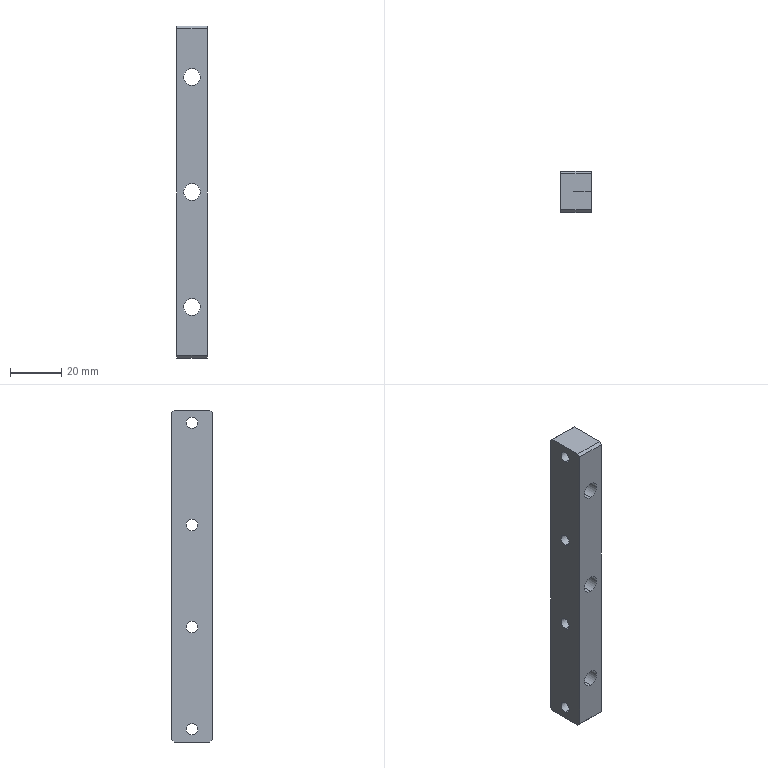Part | SolidWorks | features BaseBody 1 | 1 solid | 45 faces | box 12 x 16 x 130 mm | volume 19917 mm3 | cylinder 28 | plane 17 | commonest cylinder face diameters 4.5 x8 9 x8 6.6 x6 11 x6
STEP:
#1=CARTESIAN_POINT('',(-724.66,-691.086,-337.569));
#2=VERTEX_POINT('',#1);
#3=CARTESIAN_POINT('',(-724.66,-691.086,-333.069));
#4=VERTEX_POINT('',#3);
#5=CARTESIAN_POINT('',(-724.66,-691.086,-335.319));
#6=DIRECTION('',(-1.,0.,0.));
#7=DIRECTION('',(0.,0.,-1.));
#8=AXIS2_PLACEMENT_3D('',#5,#6,#7);
#9=CIRCLE('',#8,2.25);
#10=EDGE_CURVE('',#2,#4,#9,.T.);
#11=ORIENTED_EDGE('',*,*,#10,.T.);
#12=CARTESIAN_POINT('',(-719.66,-691.086,-333.069));
#13=VERTEX_POINT('',#12);
#14=CARTESIAN_POINT('',(-712.66,-691.086,-333.069));
#15=DIRECTION('',(1.,0.,0.));
#16=VECTOR('',#15,1000.);
#17=LINE('',#14,#16);
#18=EDGE_CURVE('',#4,#13,#17,.T.);
#19=ORIENTED_EDGE('',*,*,#18,.T.);
#20=CARTESIAN_POINT('',(-719.66,-691.086,-337.569));
#21=VERTEX_POINT('',#20);
#22=CARTESIAN_POINT('',(-719.66,-691.086,-335.319));
#23=DIRECTION('',(-1.,0.,0.));
#24=DIRECTION('',(0.,0.,-1.));
#25=AXIS2_PLACEMENT_3D('',#22,#23,#24);
#26=CIRCLE('',#25,2.25);
#27=EDGE_CURVE('',#21,#13,#26,.T.);
#28=ORIENTED_EDGE('',*,*,#27,.F.);
#29=CARTESIAN_POINT('',(-712.66,-691.086,-337.569));
#30=DIRECTION('',(1.,0.,0.));
#31=VECTOR('',#30,1000.);
#32=LINE('',#29,#31);
#33=EDGE_CURVE('',#2,#21,#32,.T.);
#34=ORIENTED_EDGE('',*,*,#33,.F.);
#35=EDGE_LOOP('',(#11,#19,#28,#34));
#36=FACE_OUTER_BOUND('',#35,.T.);
#37=CARTESIAN_POINT('',(-712.66,-691.086,-335.319));
#38=DIRECTION('',(1.,0.,0.));
#39=DIRECTION('',(0.,0.,-1.));
#40=AXIS2_PLACEMENT_3D('',#37,#38,#39);
#41=CYLINDRICAL_SURFACE('',#40,2.25);
#42=ADVANCED_FACE('',(#36),#41,.F.);
#43=CARTESIAN_POINT('',(-724.66,-691.086,-377.569));
#44=VERTEX_POINT('',#43);
#45=CARTESIAN_POINT('',(-724.66,-691.086,-373.069));
#46=VERTEX_POINT('',#45);
#47=CARTESIAN_POINT('',(-724.66,-691.086,-375.319));
#48=DIRECTION('',(-1.,0.,0.));
#49=DIRECTION('',(0.,0.,-1.));
#50=AXIS2_PLACEMENT_3D('',#47,#48,#49);
#51=CIRCLE('',#50,2.25);
#52=EDGE_CURVE('',#44,#46,#51,.T.);
#53=ORIENTED_EDGE('',*,*,#52,.T.);
#54=CARTESIAN_POINT('',(-719.66,-691.086,-373.069));
#55=VERTEX_POINT('',#54);
#56=CARTESIAN_POINT('',(-712.66,-691.086,-373.069));
#57=DIRECTION('',(1.,0.,0.));
#58=VECTOR('',#57,1000.);
#59=LINE('',#56,#58);
#60=EDGE_CURVE('',#46,#55,#59,.T.);
#61=ORIENTED_EDGE('',*,*,#60,.T.);
#62=CARTESIAN_POINT('',(-719.66,-691.086,-377.569));
#63=VERTEX_POINT('',#62);
#64=CARTESIAN_POINT('',(-719.66,-691.086,-375.319));
#65=DIRECTION('',(-1.,0.,0.));
#66=DIRECTION('',(0.,0.,-1.));
#67=AXIS2_PLACEMENT_3D('',#64,#65,#66);
#68=CIRCLE('',#67,2.25);
#69=EDGE_CURVE('',#63,#55,#68,.T.);
#70=ORIENTED_EDGE('',*,*,#69,.F.);
#71=CARTESIAN_POINT('',(-712.66,-691.086,-377.569));
#72=DIRECTION('',(1.,0.,0.));
#73=VECTOR('',#72,1000.);
#74=LINE('',#71,#73);
#75=EDGE_CURVE('',#44,#63,#74,.T.);
#76=ORIENTED_EDGE('',*,*,#75,.F.);
#77=EDGE_LOOP('',(#53,#61,#70,#76));
#78=FACE_OUTER_BOUND('',#77,.T.);
#79=CARTESIAN_POINT('',(-712.66,-691.086,-375.319));
#80=DIRECTION('',(1.,0.,0.));
#81=DIRECTION('',(0.,0.,-1.));
#82=AXIS2_PLACEMENT_3D('',#79,#80,#81);
#83=CYLINDRICAL_SURFACE('',#82,2.25);
#84=ADVANCED_FACE('',(#78),#83,.F.);
#85=CARTESIAN_POINT('',(-724.66,-691.086,-417.569));
#86=VERTEX_POINT('',#85);
#87=CARTESIAN_POINT('',(-724.66,-691.086,-413.069));
#88=VERTEX_POINT('',#87);
#89=CARTESIAN_POINT('',(-724.66,-691.086,-415.319));
#90=DIRECTION('',(-1.,0.,0.));
#91=DIRECTION('',(0.,0.,-1.));
#92=AXIS2_PLACEMENT_3D('',#89,#90,#91);
#93=CIRCLE('',#92,2.25);
#94=EDGE_CURVE('',#86,#88,#93,.T.);
#95=ORIENTED_EDGE('',*,*,#94,.T.);
#96=CARTESIAN_POINT('',(-719.66,-691.086,-413.069));
#97=VERTEX_POINT('',#96);
#98=CARTESIAN_POINT('',(-712.66,-691.086,-413.069));
#99=DIRECTION('',(1.,0.,0.));
#100=VECTOR('',#99,1000.);
#101=LINE('',#98,#100);
#102=EDGE_CURVE('',#88,#97,#101,.T.);
#103=ORIENTED_EDGE('',*,*,#102,.T.);
#104=CARTESIAN_POINT('',(-719.66,-691.086,-417.569));
#105=VERTEX_POINT('',#104);
#106=CARTESIAN_POINT('',(-719.66,-691.086,-415.319));
#107=DIRECTION('',(-1.,0.,0.));
#108=DIRECTION('',(0.,0.,-1.));
#109=AXIS2_PLACEMENT_3D('',#106,#107,#108);
#110=CIRCLE('',#109,2.25);
#111=EDGE_CURVE('',#105,#97,#110,.T.);
#112=ORIENTED_EDGE('',*,*,#111,.F.);
#113=CARTESIAN_POINT('',(-712.66,-691.086,-417.569));
#114=DIRECTION('',(1.,0.,0.));
#115=VECTOR('',#114,1000.);
#116=LINE('',#113,#115);
#117=EDGE_CURVE('',#86,#105,#116,.T.);
#118=ORIENTED_EDGE('',*,*,#117,.F.);
#119=EDGE_LOOP('',(#95,#103,#112,#118));
#120=FACE_OUTER_BOUND('',#119,.T.);
#121=CARTESIAN_POINT('',(-712.66,-691.086,-415.319));
#122=DIRECTION('',(1.,0.,0.));
#123=DIRECTION('',(0.,0.,-1.));
#124=AXIS2_PLACEMENT_3D('',#121,#122,#123);
#125=CYLINDRICAL_SURFACE('',#124,2.25);
#126=ADVANCED_FACE('',(#120),#125,.F.);
#127=CARTESIAN_POINT('',(-724.66,-691.086,-457.569));
#128=VERTEX_POINT('',#127);
#129=CARTESIAN_POINT('',(-724.66,-691.086,-453.069));
#130=VERTEX_POINT('',#129);
#131=CARTESIAN_POINT('',(-724.66,-691.086,-455.319));
#132=DIRECTION('',(-1.,0.,0.));
#133=DIRECTION('',(0.,0.,-1.));
#134=AXIS2_PLACEMENT_3D('',#131,#132,#133);
#135=CIRCLE('',#134,2.25);
#136=EDGE_CURVE('',#128,#130,#135,.T.);
#137=ORIENTED_EDGE('',*,*,#136,.T.);
#138=CARTESIAN_POINT('',(-719.66,-691.086,-453.069));
#139=VERTEX_POINT('',#138);
#140=CARTESIAN_POINT('',(-712.66,-691.086,-453.069));
#141=DIRECTION('',(1.,0.,0.));
#142=VECTOR('',#141,1000.);
#143=LINE('',#140,#142);
#144=EDGE_CURVE('',#130,#139,#143,.T.);
#145=ORIENTED_EDGE('',*,*,#144,.T.);
#146=CARTESIAN_POINT('',(-719.66,-691.086,-457.569));
#147=VERTEX_POINT('',#146);
#148=CARTESIAN_POINT('',(-719.66,-691.086,-455.319));
#149=DIRECTION('',(-1.,0.,0.));
#150=DIRECTION('',(0.,0.,-1.));
#151=AXIS2_PLACEMENT_3D('',#148,#149,#150);
#152=CIRCLE('',#151,2.25);
#153=EDGE_CURVE('',#147,#139,#152,.T.);
#154=ORIENTED_EDGE('',*,*,#153,.F.);
#155=CARTESIAN_POINT('',(-712.66,-691.086,-457.569));
#156=DIRECTION('',(1.,0.,0.));
#157=VECTOR('',#156,1000.);
#158=LINE('',#155,#157);
#159=EDGE_CURVE('',#128,#147,#158,.T.);
#160=ORIENTED_EDGE('',*,*,#159,.F.);
#161=EDGE_LOOP('',(#137,#145,#154,#160));
#162=FACE_OUTER_BOUND('',#161,.T.);
#163=CARTESIAN_POINT('',(-712.66,-691.086,-455.319));
#164=DIRECTION('',(1.,0.,0.));
#165=DIRECTION('',(0.,0.,-1.));
#166=AXIS2_PLACEMENT_3D('',#163,#164,#165);
#167=CYLINDRICAL_SURFACE('',#166,2.25);
#168=ADVANCED_FACE('',(#162),#167,.F.);
#169=CARTESIAN_POINT('',(-718.66,-690.086,-355.819));
#170=VERTEX_POINT('',#169);
#171=CARTESIAN_POINT('',(-718.66,-690.086,-344.819));
#172=VERTEX_POINT('',#171);
#173=CARTESIAN_POINT('',(-718.66,-690.086,-350.319));
#174=DIRECTION('',(0.,1.,0.));
#175=DIRECTION('',(0.,0.,1.));
#176=AXIS2_PLACEMENT_3D('',#173,#174,#175);
#177=CIRCLE('',#176,5.5);
#178=EDGE_CURVE('',#170,#172,#177,.T.);
#179=ORIENTED_EDGE('',*,*,#178,.F.);
#180=CARTESIAN_POINT('',(-718.66,-683.086,-355.819));
#181=VERTEX_POINT('',#180);
#182=CARTESIAN_POINT('',(-718.66,-683.086,-355.819));
#183=DIRECTION('',(0.,1.,0.));
#184=VECTOR('',#183,1000.);
#185=LINE('',#182,#184);
#186=EDGE_CURVE('',#170,#181,#185,.T.);
#187=ORIENTED_EDGE('',*,*,#186,.T.);
#188=CARTESIAN_POINT('',(-718.66,-683.086,-344.819));
#189=VERTEX_POINT('',#188);
#190=CARTESIAN_POINT('',(-718.66,-683.086,-350.319));
#191=DIRECTION('',(0.,1.,0.));
#192=DIRECTION('',(0.,0.,1.));
#193=AXIS2_PLACEMENT_3D('',#190,#191,#192);
#194=CIRCLE('',#193,5.5);
#195=EDGE_CURVE('',#181,#189,#194,.T.);
#196=ORIENTED_EDGE('',*,*,#195,.T.);
#197=CARTESIAN_POINT('',(-718.66,-683.086,-344.819));
#198=DIRECTION('',(0.,1.,0.));
#199=VECTOR('',#198,1000.);
#200=LINE('',#197,#199);
#201=EDGE_CURVE('',#172,#189,#200,.T.);
#202=ORIENTED_EDGE('',*,*,#201,.F.);
#203=EDGE_LOOP('',(#179,#187,#196,#202));
#204=FACE_OUTER_BOUND('',#203,.T.);
#205=CARTESIAN_POINT('',(-718.66,-683.086,-350.319));
#206=DIRECTION('',(0.,1.,0.));
#207=DIRECTION('',(0.,0.,1.));
#208=AXIS2_PLACEMENT_3D('',#205,#206,#207);
#209=CYLINDRICAL_SURFACE('',#208,5.5);
#210=ADVANCED_FACE('',(#204),#209,.F.);
#211=CARTESIAN_POINT('',(-718.66,-690.086,-400.819));
#212=VERTEX_POINT('',#211);
#213=CARTESIAN_POINT('',(-718.66,-690.086,-389.819));
#214=VERTEX_POINT('',#213);
#215=CARTESIAN_POINT('',(-718.66,-690.086,-395.319));
#216=DIRECTION('',(0.,1.,0.));
#217=DIRECTION('',(0.,0.,1.));
#218=AXIS2_PLACEMENT_3D('',#215,#216,#217);
#219=CIRCLE('',#218,5.5);
#220=EDGE_CURVE('',#212,#214,#219,.T.);
#221=ORIENTED_EDGE('',*,*,#220,.F.);
#222=CARTESIAN_POINT('',(-718.66,-683.086,-400.819));
#223=VERTEX_POINT('',#222);
#224=CARTESIAN_POINT('',(-718.66,-683.086,-400.819));
#225=DIRECTION('',(0.,1.,0.));
#226=VECTOR('',#225,1000.);
#227=LINE('',#224,#226);
#228=EDGE_CURVE('',#212,#223,#227,.T.);
#229=ORIENTED_EDGE('',*,*,#228,.T.);
#230=CARTESIAN_POINT('',(-718.66,-683.086,-389.819));
#231=VERTEX_POINT('',#230);
#232=CARTESIAN_POINT('',(-718.66,-683.086,-395.319));
#233=DIRECTION('',(0.,1.,0.));
#234=DIRECTION('',(0.,0.,1.));
#235=AXIS2_PLACEMENT_3D('',#232,#233,#234);
#236=CIRCLE('',#235,5.5);
#237=EDGE_CURVE('',#223,#231,#236,.T.);
#238=ORIENTED_EDGE('',*,*,#237,.T.);
#239=CARTESIAN_POINT('',(-718.66,-683.086,-389.819));
#240=DIRECTION('',(0.,1.,0.));
#241=VECTOR('',#240,1000.);
#242=LINE('',#239,#241);
#243=EDGE_CURVE('',#214,#231,#242,.T.);
#244=ORIENTED_EDGE('',*,*,#243,.F.);
#245=EDGE_LOOP('',(#221,#229,#238,#244));
#246=FACE_OUTER_BOUND('',#245,.T.);
#247=CARTESIAN_POINT('',(-718.66,-683.086,-395.319));
#248=DIRECTION('',(0.,1.,0.));
#249=DIRECTION('',(0.,0.,1.));
#250=AXIS2_PLACEMENT_3D('',#247,#248,#249);
#251=CYLINDRICAL_SURFACE('',#250,5.5);
#252=ADVANCED_FACE('',(#246),#251,.F.);
#253=CARTESIAN_POINT('',(-718.66,-690.086,-445.819));
#254=VERTEX_POINT('',#253);
#255=CARTESIAN_POINT('',(-718.66,-690.086,-434.819));
#256=VERTEX_POINT('',#255);
#257=CARTESIAN_POINT('',(-718.66,-690.086,-440.319));
#258=DIRECTION('',(0.,1.,0.));
#259=DIRECTION('',(0.,0.,1.));
#260=AXIS2_PLACEMENT_3D('',#257,#258,#259);
#261=CIRCLE('',#260,5.5);
#262=EDGE_CURVE('',#254,#256,#261,.T.);
#263=ORIENTED_EDGE('',*,*,#262,.F.);
#264=CARTESIAN_POINT('',(-718.66,-683.086,-445.819));
#265=VERTEX_POINT('',#264);
#266=CARTESIAN_POINT('',(-718.66,-683.086,-445.819));
#267=DIRECTION('',(0.,1.,0.));
#268=VECTOR('',#267,1000.);
#269=LINE('',#266,#268);
#270=EDGE_CURVE('',#254,#265,#269,.T.);
#271=ORIENTED_EDGE('',*,*,#270,.T.);
#272=CARTESIAN_POINT('',(-718.66,-683.086,-434.819));
#273=VERTEX_POINT('',#272);
#274=CARTESIAN_POINT('',(-718.66,-683.086,-440.319));
#275=DIRECTION('',(0.,1.,0.));
#276=DIRECTION('',(0.,0.,1.));
#277=AXIS2_PLACEMENT_3D('',#274,#275,#276);
#278=CIRCLE('',#277,5.5);
#279=EDGE_CURVE('',#265,#273,#278,.T.);
#280=ORIENTED_EDGE('',*,*,#279,.T.);
#281=CARTESIAN_POINT('',(-718.66,-683.086,-434.819));
#282=DIRECTION('',(0.,1.,0.));
#283=VECTOR('',#282,1000.);
#284=LINE('',#281,#283);
#285=EDGE_CURVE('',#256,#273,#284,.T.);
#286=ORIENTED_EDGE('',*,*,#285,.F.);
#287=EDGE_LOOP('',(#263,#271,#280,#286));
#288=FACE_OUTER_BOUND('',#287,.T.);
#289=CARTESIAN_POINT('',(-718.66,-683.086,-440.319));
#290=DIRECTION('',(0.,1.,0.));
#291=DIRECTION('',(0.,0.,1.));
#292=AXIS2_PLACEMENT_3D('',#289,#290,#291);
#293=CYLINDRICAL_SURFACE('',#292,5.5);
#294=ADVANCED_FACE('',(#288),#293,.F.);
#295=CARTESIAN_POINT('',(-718.66,-699.086,-347.019));
#296=VERTEX_POINT('',#295);
#297=CARTESIAN_POINT('',(-718.66,-699.086,-353.619));
#298=VERTEX_POINT('',#297);
#299=CARTESIAN_POINT('',(-718.66,-699.086,-350.319));
#300=DIRECTION('',(0.,-1.,0.));
#301=DIRECTION('',(0.,0.,1.));
#302=AXIS2_PLACEMENT_3D('',#299,#300,#301);
#303=CIRCLE('',#302,3.3);
#304=EDGE_CURVE('',#296,#298,#303,.T.);
#305=ORIENTED_EDGE('',*,*,#304,.T.);
#306=CARTESIAN_POINT('',(-718.66,-690.086,-353.619));
#307=VERTEX_POINT('',#306);
#308=CARTESIAN_POINT('',(-718.66,-683.086,-353.619));
#309=DIRECTION('',(0.,1.,0.));
#310=VECTOR('',#309,1000.);
#311=LINE('',#308,#310);
#312=EDGE_CURVE('',#298,#307,#311,.T.);
#313=ORIENTED_EDGE('',*,*,#312,.T.);
#314=CARTESIAN_POINT('',(-718.66,-690.086,-347.019));
#315=VERTEX_POINT('',#314);
#316=CARTESIAN_POINT('',(-718.66,-690.086,-350.319));
#317=DIRECTION('',(0.,-1.,0.));
#318=DIRECTION('',(0.,0.,1.));
#319=AXIS2_PLACEMENT_3D('',#316,#317,#318);
#320=CIRCLE('',#319,3.3);
#321=EDGE_CURVE('',#315,#307,#320,.T.);
#322=ORIENTED_EDGE('',*,*,#321,.F.);
#323=CARTESIAN_POINT('',(-718.66,-683.086,-347.019));
#324=DIRECTION('',(0.,1.,0.));
#325=VECTOR('',#324,1000.);
#326=LINE('',#323,#325);
#327=EDGE_CURVE('',#296,#315,#326,.T.);
#328=ORIENTED_EDGE('',*,*,#327,.F.);
#329=EDGE_LOOP('',(#305,#313,#322,#328));
#330=FACE_OUTER_BOUND('',#329,.T.);
#331=CARTESIAN_POINT('',(-718.66,-683.086,-350.319));
#332=DIRECTION('',(0.,1.,0.));
#333=DIRECTION('',(0.,0.,1.));
#334=AXIS2_PLACEMENT_3D('',#331,#332,#333);
#335=CYLINDRICAL_SURFACE('',#334,3.3);
#336=ADVANCED_FACE('',(#330),#335,.F.);
#337=CARTESIAN_POINT('',(-718.66,-699.086,-392.019));
#338=VERTEX_POINT('',#337);
#339=CARTESIAN_POINT('',(-718.66,-699.086,-398.619));
#340=VERTEX_POINT('',#339);
#341=CARTESIAN_POINT('',(-718.66,-699.086,-395.319));
#342=DIRECTION('',(0.,-1.,0.));
#343=DIRECTION('',(0.,0.,1.));
#344=AXIS2_PLACEMENT_3D('',#341,#342,#343);
#345=CIRCLE('',#344,3.3);
#346=EDGE_CURVE('',#338,#340,#345,.T.);
#347=ORIENTED_EDGE('',*,*,#346,.T.);
#348=CARTESIAN_POINT('',(-718.66,-690.086,-398.619));
#349=VERTEX_POINT('',#348);
#350=CARTESIAN_POINT('',(-718.66,-683.086,-398.619));
#351=DIRECTION('',(0.,1.,0.));
#352=VECTOR('',#351,1000.);
#353=LINE('',#350,#352);
#354=EDGE_CURVE('',#340,#349,#353,.T.);
#355=ORIENTED_EDGE('',*,*,#354,.T.);
#356=CARTESIAN_POINT('',(-718.66,-690.086,-392.019));
#357=VERTEX_POINT('',#356);
#358=CARTESIAN_POINT('',(-718.66,-690.086,-395.319));
#359=DIRECTION('',(0.,-1.,0.));
#360=DIRECTION('',(0.,0.,1.));
#361=AXIS2_PLACEMENT_3D('',#358,#359,#360);
#362=CIRCLE('',#361,3.3);
#363=EDGE_CURVE('',#357,#349,#362,.T.);
#364=ORIENTED_EDGE('',*,*,#363,.F.);
#365=CARTESIAN_POINT('',(-718.66,-683.086,-392.019));
#366=DIRECTION('',(0.,1.,0.));
#367=VECTOR('',#366,1000.);
#368=LINE('',#365,#367);
#369=EDGE_CURVE('',#338,#357,#368,.T.);
#370=ORIENTED_EDGE('',*,*,#369,.F.);
#371=EDGE_LOOP('',(#347,#355,#364,#370));
#372=FACE_OUTER_BOUND('',#371,.T.);
#373=CARTESIAN_POINT('',(-718.66,-683.086,-395.319));
#374=DIRECTION('',(0.,1.,0.));
#375=DIRECTION('',(0.,0.,1.));
#376=AXIS2_PLACEMENT_3D('',#373,#374,#375);
#377=CYLINDRICAL_SURFACE('',#376,3.3);
#378=ADVANCED_FACE('',(#372),#377,.F.);
#379=CARTESIAN_POINT('',(-718.66,-699.086,-437.019));
#380=VERTEX_POINT('',#379);
#381=CARTESIAN_POINT('',(-718.66,-699.086,-443.619));
#382=VERTEX_POINT('',#381);
#383=CARTESIAN_POINT('',(-718.66,-699.086,-440.319));
#384=DIRECTION('',(0.,-1.,0.));
#385=DIRECTION('',(0.,0.,1.));
#386=AXIS2_PLACEMENT_3D('',#383,#384,#385);
#387=CIRCLE('',#386,3.3);
#388=EDGE_CURVE('',#380,#382,#387,.T.);
#389=ORIENTED_EDGE('',*,*,#388,.T.);
#390=CARTESIAN_POINT('',(-718.66,-690.086,-443.619));
#391=VERTEX_POINT('',#390);
#392=CARTESIAN_POINT('',(-718.66,-683.086,-443.619));
#393=DIRECTION('',(0.,1.,0.));
#394=VECTOR('',#393,1000.);
#395=LINE('',#392,#394);
#396=EDGE_CURVE('',#382,#391,#395,.T.);
#397=ORIENTED_EDGE('',*,*,#396,.T.);
#398=CARTESIAN_POINT('',(-718.66,-690.086,-437.019));
#399=VERTEX_POINT('',#398);
#400=CARTESIAN_POINT('',(-718.66,-690.086,-440.319));
#401=DIRECTION('',(0.,-1.,0.));
#402=DIRECTION('',(0.,0.,1.));
#403=AXIS2_PLACEMENT_3D('',#400,#401,#402);
#404=CIRCLE('',#403,3.3);
#405=EDGE_CURVE('',#399,#391,#404,.T.);
#406=ORIENTED_EDGE('',*,*,#405,.F.);
#407=CARTESIAN_POINT('',(-718.66,-683.086,-437.019));
#408=DIRECTION('',(0.,1.,0.));
#409=VECTOR('',#408,1000.);
#410=LINE('',#407,#409);
#411=EDGE_CURVE('',#380,#399,#410,.T.);
#412=ORIENTED_EDGE('',*,*,#411,.F.);
#413=EDGE_LOOP('',(#389,#397,#406,#412));
#414=FACE_OUTER_BOUND('',#413,.T.);
#415=CARTESIAN_POINT('',(-718.66,-683.086,-440.319));
#416=DIRECTION('',(0.,1.,0.));
#417=DIRECTION('',(0.,0.,1.));
#418=AXIS2_PLACEMENT_3D('',#415,#416,#417);
#419=CYLINDRICAL_SURFACE('',#418,3.3);
#420=ADVANCED_FACE('',(#414),#419,.F.);
#421=CARTESIAN_POINT('',(-719.66,-691.086,-339.819));
#422=VERTEX_POINT('',#421);
#423=CARTESIAN_POINT('',(-719.66,-691.086,-330.819));
#424=VERTEX_POINT('',#423);
#425=CARTESIAN_POINT('',(-719.66,-691.086,-335.319));
#426=DIRECTION('',(-1.,0.,0.));
#427=DIRECTION('',(0.,0.,-1.));
#428=AXIS2_PLACEMENT_3D('',#425,#426,#427);
#429=CIRCLE('',#428,4.5);
#430=EDGE_CURVE('',#422,#424,#429,.T.);
#431=ORIENTED_EDGE('',*,*,#430,.T.);
#432=CARTESIAN_POINT('',(-712.66,-691.086,-330.819));
#433=VERTEX_POINT('',#432);
#434=CARTESIAN_POINT('',(-712.66,-691.086,-330.819));
#435=DIRECTION('',(1.,0.,0.));
#436=VECTOR('',#435,1000.);
#437=LINE('',#434,#436);
#438=EDGE_CURVE('',#424,#433,#437,.T.);
#439=ORIENTED_EDGE('',*,*,#438,.T.);
#440=CARTESIAN_POINT('',(-712.66,-691.086,-339.819));
#441=VERTEX_POINT('',#440);
#442=CARTESIAN_POINT('',(-712.66,-691.086,-335.319));
#443=DIRECTION('',(-1.,0.,0.));
#444=DIRECTION('',(0.,0.,-1.));
#445=AXIS2_PLACEMENT_3D('',#442,#443,#444);
#446=CIRCLE('',#445,4.5);
#447=EDGE_CURVE('',#441,#433,#446,.T.);
#448=ORIENTED_EDGE('',*,*,#447,.F.);
#449=CARTESIAN_POINT('',(-712.66,-691.086,-339.819));
#450=DIRECTION('',(1.,0.,0.));
#451=VECTOR('',#450,1000.);
#452=LINE('',#449,#451);
#453=EDGE_CURVE('',#422,#441,#452,.T.);
#454=ORIENTED_EDGE('',*,*,#453,.F.);
#455=EDGE_LOOP('',(#431,#439,#448,#454));
#456=FACE_OUTER_BOUND('',#455,.T.);
#457=CARTESIAN_POINT('',(-712.66,-691.086,-335.319));
#458=DIRECTION('',(1.,0.,0.));
#459=DIRECTION('',(0.,0.,-1.));
#460=AXIS2_PLACEMENT_3D('',#457,#458,#459);
#461=CYLINDRICAL_SURFACE('',#460,4.5);
#462=ADVANCED_FACE('',(#456),#461,.F.);
#463=CARTESIAN_POINT('',(-719.66,-691.086,-379.819));
#464=VERTEX_POINT('',#463);
#465=CARTESIAN_POINT('',(-719.66,-691.086,-370.819));
#466=VERTEX_POINT('',#465);
#467=CARTESIAN_POINT('',(-719.66,-691.086,-375.319));
#468=DIRECTION('',(-1.,0.,0.));
#469=DIRECTION('',(0.,0.,-1.));
#470=AXIS2_PLACEMENT_3D('',#467,#468,#469);
#471=CIRCLE('',#470,4.5);
#472=EDGE_CURVE('',#464,#466,#471,.T.);
#473=ORIENTED_EDGE('',*,*,#472,.T.);
#474=CARTESIAN_POINT('',(-712.66,-691.086,-370.819));
#475=VERTEX_POINT('',#474);
#476=CARTESIAN_POINT('',(-712.66,-691.086,-370.819));
#477=DIRECTION('',(1.,0.,0.));
#478=VECTOR('',#477,1000.);
#479=LINE('',#476,#478);
#480=EDGE_CURVE('',#466,#475,#479,.T.);
#481=ORIENTED_EDGE('',*,*,#480,.T.);
#482=CARTESIAN_POINT('',(-712.66,-691.086,-379.819));
#483=VERTEX_POINT('',#482);
#484=CARTESIAN_POINT('',(-712.66,-691.086,-375.319));
#485=DIRECTION('',(-1.,0.,0.));
#486=DIRECTION('',(0.,0.,-1.));
#487=AXIS2_PLACEMENT_3D('',#484,#485,#486);
#488=CIRCLE('',#487,4.5);
#489=EDGE_CURVE('',#483,#475,#488,.T.);
#490=ORIENTED_EDGE('',*,*,#489,.F.);
#491=CARTESIAN_POINT('',(-712.66,-691.086,-379.819));
#492=DIRECTION('',(1.,0.,0.));
#493=VECTOR('',#492,1000.);
#494=LINE('',#491,#493);
#495=EDGE_CURVE('',#464,#483,#494,.T.);
#496=ORIENTED_EDGE('',*,*,#495,.F.);
#497=EDGE_LOOP('',(#473,#481,#490,#496));
#498=FACE_OUTER_BOUND('',#497,.T.);
#499=CARTESIAN_POINT('',(-712.66,-691.086,-375.319));
#500=DIRECTION('',(1.,0.,0.));
#501=DIRECTION('',(0.,0.,-1.));
#502=AXIS2_PLACEMENT_3D('',#499,#500,#501);
#503=CYLINDRICAL_SURFACE('',#502,4.5);
#504=ADVANCED_FACE('',(#498),#503,.F.);
#505=CARTESIAN_POINT('',(-719.66,-691.086,-419.819));
#506=VERTEX_POINT('',#505);
#507=CARTESIAN_POINT('',(-719.66,-691.086,-410.819));
#508=VERTEX_POINT('',#507);
#509=CARTESIAN_POINT('',(-719.66,-691.086,-415.319));
#510=DIRECTION('',(-1.,0.,0.));
#511=DIRECTION('',(0.,0.,-1.));
#512=AXIS2_PLACEMENT_3D('',#509,#510,#511);
#513=CIRCLE('',#512,4.5);
#514=EDGE_CURVE('',#506,#508,#513,.T.);
#515=ORIENTED_EDGE('',*,*,#514,.T.);
#516=CARTESIAN_POINT('',(-712.66,-691.086,-410.819));
#517=VERTEX_POINT('',#516);
#518=CARTESIAN_POINT('',(-712.66,-691.086,-410.819));
#519=DIRECTION('',(1.,0.,0.));
#520=VECTOR('',#519,1000.);
#521=LINE('',#518,#520);
#522=EDGE_CURVE('',#508,#517,#521,.T.);
#523=ORIENTED_EDGE('',*,*,#522,.T.);
#524=CARTESIAN_POINT('',(-712.66,-691.086,-419.819));
#525=VERTEX_POINT('',#524);
#526=CARTESIAN_POINT('',(-712.66,-691.086,-415.319));
#527=DIRECTION('',(-1.,0.,0.));
#528=DIRECTION('',(0.,0.,-1.));
#529=AXIS2_PLACEMENT_3D('',#526,#527,#528);
#530=CIRCLE('',#529,4.5);
#531=EDGE_CURVE('',#525,#517,#530,.T.);
#532=ORIENTED_EDGE('',*,*,#531,.F.);
#533=CARTESIAN_POINT('',(-712.66,-691.086,-419.819));
#534=DIRECTION('',(1.,0.,0.));
#535=VECTOR('',#534,1000.);
#536=LINE('',#533,#535);
#537=EDGE_CURVE('',#506,#525,#536,.T.);
#538=ORIENTED_EDGE('',*,*,#537,.F.);
#539=EDGE_LOOP('',(#515,#523,#532,#538));
#540=FACE_OUTER_BOUND('',#539,.T.);
#541=CARTESIAN_POINT('',(-712.66,-691.086,-415.319));
#542=DIRECTION('',(1.,0.,0.));
#543=DIRECTION('',(0.,0.,-1.));
#544=AXIS2_PLACEMENT_3D('',#541,#542,#543);
#545=CYLINDRICAL_SURFACE('',#544,4.5);
#546=ADVANCED_FACE('',(#540),#545,.F.);
#547=CARTESIAN_POINT('',(-719.66,-691.086,-459.819));
#548=VERTEX_POINT('',#547);
#549=CARTESIAN_POINT('',(-719.66,-691.086,-450.819));
#550=VERTEX_POINT('',#549);
#551=CARTESIAN_POINT('',(-719.66,-691.086,-455.319));
#552=DIRECTION('',(-1.,0.,0.));
#553=DIRECTION('',(0.,0.,-1.));
#554=AXIS2_PLACEMENT_3D('',#551,#552,#553);
#555=CIRCLE('',#554,4.5);
#556=EDGE_CURVE('',#548,#550,#555,.T.);
#557=ORIENTED_EDGE('',*,*,#556,.T.);
#558=CARTESIAN_POINT('',(-712.66,-691.086,-450.819));
#559=VERTEX_POINT('',#558);
#560=CARTESIAN_POINT('',(-712.66,-691.086,-450.819));
#561=DIRECTION('',(1.,0.,0.));
#562=VECTOR('',#561,1000.);
#563=LINE('',#560,#562);
#564=EDGE_CURVE('',#550,#559,#563,.T.);
#565=ORIENTED_EDGE('',*,*,#564,.T.);
#566=CARTESIAN_POINT('',(-712.66,-691.086,-459.819));
#567=VERTEX_POINT('',#566);
#568=CARTESIAN_POINT('',(-712.66,-691.086,-455.319));
#569=DIRECTION('',(-1.,0.,0.));
#570=DIRECTION('',(0.,0.,-1.));
#571=AXIS2_PLACEMENT_3D('',#568,#569,#570);
#572=CIRCLE('',#571,4.5);
#573=EDGE_CURVE('',#567,#559,#572,.T.);
#574=ORIENTED_EDGE('',*,*,#573,.F.);
#575=CARTESIAN_POINT('',(-712.66,-691.086,-459.819));
#576=DIRECTION('',(1.,0.,0.));
#577=VECTOR('',#576,1000.);
#578=LINE('',#575,#577);
#579=EDGE_CURVE('',#548,#567,#578,.T.);
#580=ORIENTED_EDGE('',*,*,#579,.F.);
#581=EDGE_LOOP('',(#557,#565,#574,#580));
#582=FACE_OUTER_BOUND('',#581,.T.);
#583=CARTESIAN_POINT('',(-712.66,-691.086,-455.319));
#584=DIRECTION('',(1.,0.,0.));
#585=DIRECTION('',(0.,0.,-1.));
#586=AXIS2_PLACEMENT_3D('',#583,#584,#585);
#587=CYLINDRICAL_SURFACE('',#586,4.5);
#588=ADVANCED_FACE('',(#582),#587,.F.);
#589=ORIENTED_EDGE('',*,*,#10,.F.);
#590=CARTESIAN_POINT('',(-724.66,-691.086,-335.319));
#591=DIRECTION('',(-1.,0.,0.));
#592=DIRECTION('',(0.,0.,-1.));
#593=AXIS2_PLACEMENT_3D('',#590,#591,#592);
#594=CIRCLE('',#593,2.25);
#595=EDGE_CURVE('',#4,#2,#594,.T.);
#596=ORIENTED_EDGE('',*,*,#595,.F.);
#597=EDGE_LOOP('',(#589,#596));
#598=FACE_BOUND('',#597,.T.);
#599=ORIENTED_EDGE('',*,*,#52,.F.);
#600=CARTESIAN_POINT('',(-724.66,-691.086,-375.319));
#601=DIRECTION('',(-1.,0.,0.));
#602=DIRECTION('',(0.,0.,-1.));
#603=AXIS2_PLACEMENT_3D('',#600,#601,#602);
#604=CIRCLE('',#603,2.25);
#605=EDGE_CURVE('',#46,#44,#604,.T.);
#606=ORIENTED_EDGE('',*,*,#605,.F.);
#607=EDGE_LOOP('',(#599,#606));
#608=FACE_BOUND('',#607,.T.);
#609=ORIENTED_EDGE('',*,*,#94,.F.);
#610=CARTESIAN_POINT('',(-724.66,-691.086,-415.319));
#611=DIRECTION('',(-1.,0.,0.));
#612=DIRECTION('',(0.,0.,-1.));
#613=AXIS2_PLACEMENT_3D('',#610,#611,#612);
#614=CIRCLE('',#613,2.25);
#615=EDGE_CURVE('',#88,#86,#614,.T.);
#616=ORIENTED_EDGE('',*,*,#615,.F.);
#617=EDGE_LOOP('',(#609,#616));
#618=FACE_BOUND('',#617,.T.);
#619=ORIENTED_EDGE('',*,*,#136,.F.);
#620=CARTESIAN_POINT('',(-724.66,-691.086,-455.319));
#621=DIRECTION('',(-1.,0.,0.));
#622=DIRECTION('',(0.,0.,-1.));
#623=AXIS2_PLACEMENT_3D('',#620,#621,#622);
#624=CIRCLE('',#623,2.25);
#625=EDGE_CURVE('',#130,#128,#624,.T.);
#626=ORIENTED_EDGE('',*,*,#625,.F.);
#627=EDGE_LOOP('',(#619,#626));
#628=FACE_BOUND('',#627,.T.);
#629=CARTESIAN_POINT('',(-724.66,-683.086,-459.319));
#630=VERTEX_POINT('',#629);
#631=CARTESIAN_POINT('',(-724.66,-683.086,-331.319));
#632=VERTEX_POINT('',#631);
#633=CARTESIAN_POINT('',(-724.66,-683.086,-395.319));
#634=DIRECTION('',(0.,0.,1.));
#635=VECTOR('',#634,1000.);
#636=LINE('',#633,#635);
#637=EDGE_CURVE('',#630,#632,#636,.T.);
#638=ORIENTED_EDGE('',*,*,#637,.F.);
#639=CARTESIAN_POINT('',(-724.66,-684.086,-460.319));
#640=VERTEX_POINT('',#639);
#641=CARTESIAN_POINT('',(-724.66,-683.086,-459.319));
#642=DIRECTION('',(0.,-0.7071,-0.7071));
#643=VECTOR('',#642,1000.);
#644=LINE('',#641,#643);
#645=EDGE_CURVE('',#630,#640,#644,.T.);
#646=ORIENTED_EDGE('',*,*,#645,.T.);
#647=CARTESIAN_POINT('',(-724.66,-698.086,-460.319));
#648=VERTEX_POINT('',#647);
#649=CARTESIAN_POINT('',(-724.66,-691.086,-460.319));
#650=DIRECTION('',(0.,1.,0.));
#651=VECTOR('',#650,1000.);
#652=LINE('',#649,#651);
#653=EDGE_CURVE('',#648,#640,#652,.T.);
#654=ORIENTED_EDGE('',*,*,#653,.F.);
#655=CARTESIAN_POINT('',(-724.66,-699.086,-459.319));
#656=VERTEX_POINT('',#655);
#657=CARTESIAN_POINT('',(-724.66,-698.086,-460.319));
#658=DIRECTION('',(0.,-0.7071,0.7071));
#659=VECTOR('',#658,1000.);
#660=LINE('',#657,#659);
#661=EDGE_CURVE('',#648,#656,#660,.T.);
#662=ORIENTED_EDGE('',*,*,#661,.T.);
#663=CARTESIAN_POINT('',(-724.66,-699.086,-331.319));
#664=VERTEX_POINT('',#663);
#665=CARTESIAN_POINT('',(-724.66,-699.086,-395.319));
#666=DIRECTION('',(0.,0.,-1.));
#667=VECTOR('',#666,1000.);
#668=LINE('',#665,#667);
#669=EDGE_CURVE('',#664,#656,#668,.T.);
#670=ORIENTED_EDGE('',*,*,#669,.F.);
#671=CARTESIAN_POINT('',(-724.66,-698.086,-330.319));
#672=VERTEX_POINT('',#671);
#673=CARTESIAN_POINT('',(-724.66,-699.086,-331.319));
#674=DIRECTION('',(0.,0.7071,0.7071));
#675=VECTOR('',#674,1000.);
#676=LINE('',#673,#675);
#677=EDGE_CURVE('',#664,#672,#676,.T.);
#678=ORIENTED_EDGE('',*,*,#677,.T.);
#679=CARTESIAN_POINT('',(-724.66,-684.086,-330.319));
#680=VERTEX_POINT('',#679);
#681=CARTESIAN_POINT('',(-724.66,-691.086,-330.319));
#682=DIRECTION('',(0.,-1.,0.));
#683=VECTOR('',#682,1000.);
#684=LINE('',#681,#683);
#685=EDGE_CURVE('',#680,#672,#684,.T.);
#686=ORIENTED_EDGE('',*,*,#685,.F.);
#687=CARTESIAN_POINT('',(-724.66,-684.086,-330.319));
#688=DIRECTION('',(0.,0.7071,-0.7071));
#689=VECTOR('',#688,1000.);
#690=LINE('',#687,#689);
#691=EDGE_CURVE('',#680,#632,#690,.T.);
#692=ORIENTED_EDGE('',*,*,#691,.T.);
#693=EDGE_LOOP('',(#638,#646,#654,#662,#670,#678,#686,#692));
#694=FACE_OUTER_BOUND('',#693,.T.);
#695=CARTESIAN_POINT('',(-724.66,-691.086,-395.319));
#696=DIRECTION('',(1.,0.,0.));
#697=DIRECTION('',(0.,0.,-1.));
#698=AXIS2_PLACEMENT_3D('',#695,#696,#697);
#699=PLANE('',#698);
#700=ADVANCED_FACE('',(#598,#608,#618,#628,#694),#699,.F.);
#701=ORIENTED_EDGE('',*,*,#18,.F.);
#702=ORIENTED_EDGE('',*,*,#595,.T.);
#703=ORIENTED_EDGE('',*,*,#33,.T.);
#704=CARTESIAN_POINT('',(-719.66,-691.086,-335.319));
#705=DIRECTION('',(-1.,0.,0.));
#706=DIRECTION('',(0.,0.,-1.));
#707=AXIS2_PLACEMENT_3D('',#704,#705,#706);
#708=CIRCLE('',#707,2.25);
#709=EDGE_CURVE('',#13,#21,#708,.T.);
#710=ORIENTED_EDGE('',*,*,#709,.F.);
#711=EDGE_LOOP('',(#701,#702,#703,#710));
#712=FACE_OUTER_BOUND('',#711,.T.);
#713=CARTESIAN_POINT('',(-712.66,-691.086,-335.319));
#714=DIRECTION('',(1.,0.,0.));
#715=DIRECTION('',(0.,0.,-1.));
#716=AXIS2_PLACEMENT_3D('',#713,#714,#715);
#717=CYLINDRICAL_SURFACE('',#716,2.25);
#718=ADVANCED_FACE('',(#712),#717,.F.);
#719=ORIENTED_EDGE('',*,*,#60,.F.);
#720=ORIENTED_EDGE('',*,*,#605,.T.);
#721=ORIENTED_EDGE('',*,*,#75,.T.);
#722=CARTESIAN_POINT('',(-719.66,-691.086,-375.319));
#723=DIRECTION('',(-1.,0.,0.));
#724=DIRECTION('',(0.,0.,-1.));
#725=AXIS2_PLACEMENT_3D('',#722,#723,#724);
#726=CIRCLE('',#725,2.25);
#727=EDGE_CURVE('',#55,#63,#726,.T.);
#728=ORIENTED_EDGE('',*,*,#727,.F.);
#729=EDGE_LOOP('',(#719,#720,#721,#728));
#730=FACE_OUTER_BOUND('',#729,.T.);
#731=CARTESIAN_POINT('',(-712.66,-691.086,-375.319));
#732=DIRECTION('',(1.,0.,0.));
#733=DIRECTION('',(0.,0.,-1.));
#734=AXIS2_PLACEMENT_3D('',#731,#732,#733);
#735=CYLINDRICAL_SURFACE('',#734,2.25);
#736=ADVANCED_FACE('',(#730),#735,.F.);
#737=ORIENTED_EDGE('',*,*,#102,.F.);
#738=ORIENTED_EDGE('',*,*,#615,.T.);
#739=ORIENTED_EDGE('',*,*,#117,.T.);
#740=CARTESIAN_POINT('',(-719.66,-691.086,-415.319));
#741=DIRECTION('',(-1.,0.,0.));
#742=DIRECTION('',(0.,0.,-1.));
#743=AXIS2_PLACEMENT_3D('',#740,#741,#742);
#744=CIRCLE('',#743,2.25);
#745=EDGE_CURVE('',#97,#105,#744,.T.);
#746=ORIENTED_EDGE('',*,*,#745,.F.);
#747=EDGE_LOOP('',(#737,#738,#739,#746));
#748=FACE_OUTER_BOUND('',#747,.T.);
#749=CARTESIAN_POINT('',(-712.66,-691.086,-415.319));
#750=DIRECTION('',(1.,0.,0.));
#751=DIRECTION('',(0.,0.,-1.));
#752=AXIS2_PLACEMENT_3D('',#749,#750,#751);
#753=CYLINDRICAL_SURFACE('',#752,2.25);
#754=ADVANCED_FACE('',(#748),#753,.F.);
#755=ORIENTED_EDGE('',*,*,#144,.F.);
#756=ORIENTED_EDGE('',*,*,#625,.T.);
#757=ORIENTED_EDGE('',*,*,#159,.T.);
#758=CARTESIAN_POINT('',(-719.66,-691.086,-455.319));
#759=DIRECTION('',(-1.,0.,0.));
#760=DIRECTION('',(0.,0.,-1.));
#761=AXIS2_PLACEMENT_3D('',#758,#759,#760);
#762=CIRCLE('',#761,2.25);
#763=EDGE_CURVE('',#139,#147,#762,.T.);
#764=ORIENTED_EDGE('',*,*,#763,.F.);
#765=EDGE_LOOP('',(#755,#756,#757,#764));
#766=FACE_OUTER_BOUND('',#765,.T.);
#767=CARTESIAN_POINT('',(-712.66,-691.086,-455.319));
#768=DIRECTION('',(1.,0.,0.));
#769=DIRECTION('',(0.,0.,-1.));
#770=AXIS2_PLACEMENT_3D('',#767,#768,#769);
#771=CYLINDRICAL_SURFACE('',#770,2.25);
#772=ADVANCED_FACE('',(#766),#771,.F.);
#773=CARTESIAN_POINT('',(-718.66,-683.086,-350.319));
#774=DIRECTION('',(0.,1.,0.));
#775=DIRECTION('',(0.,0.,1.));
#776=AXIS2_PLACEMENT_3D('',#773,#774,#775);
#777=CIRCLE('',#776,5.5);
#778=EDGE_CURVE('',#189,#181,#777,.T.);
#779=ORIENTED_EDGE('',*,*,#778,.F.);
#780=ORIENTED_EDGE('',*,*,#195,.F.);
#781=EDGE_LOOP('',(#779,#780));
#782=FACE_BOUND('',#781,.T.);
#783=CARTESIAN_POINT('',(-718.66,-683.086,-395.319));
#784=DIRECTION('',(0.,1.,0.));
#785=DIRECTION('',(0.,0.,1.));
#786=AXIS2_PLACEMENT_3D('',#783,#784,#785);
#787=CIRCLE('',#786,5.5);
#788=EDGE_CURVE('',#231,#223,#787,.T.);
#789=ORIENTED_EDGE('',*,*,#788,.F.);
#790=ORIENTED_EDGE('',*,*,#237,.F.);
#791=EDGE_LOOP('',(#789,#790));
#792=FACE_BOUND('',#791,.T.);
#793=CARTESIAN_POINT('',(-718.66,-683.086,-440.319));
#794=DIRECTION('',(0.,1.,0.));
#795=DIRECTION('',(0.,0.,1.));
#796=AXIS2_PLACEMENT_3D('',#793,#794,#795);
#797=CIRCLE('',#796,5.5);
#798=EDGE_CURVE('',#273,#265,#797,.T.);
#799=ORIENTED_EDGE('',*,*,#798,.F.);
#800=ORIENTED_EDGE('',*,*,#279,.F.);
#801=EDGE_LOOP('',(#799,#800));
#802=FACE_BOUND('',#801,.T.);
#803=ORIENTED_EDGE('',*,*,#637,.T.);
#804=CARTESIAN_POINT('',(-712.66,-683.086,-331.319));
#805=VERTEX_POINT('',#804);
#806=CARTESIAN_POINT('',(-712.66,-683.086,-331.319));
#807=DIRECTION('',(-1.,0.,0.));
#808=VECTOR('',#807,1000.);
#809=LINE('',#806,#808);
#810=EDGE_CURVE('',#805,#632,#809,.T.);
#811=ORIENTED_EDGE('',*,*,#810,.F.);
#812=CARTESIAN_POINT('',(-712.66,-683.086,-459.319));
#813=VERTEX_POINT('',#812);
#814=CARTESIAN_POINT('',(-712.66,-683.086,-330.319));
#815=DIRECTION('',(0.,0.,1.));
#816=VECTOR('',#815,1000.);
#817=LINE('',#814,#816);
#818=EDGE_CURVE('',#813,#805,#817,.T.);
#819=ORIENTED_EDGE('',*,*,#818,.F.);
#820=CARTESIAN_POINT('',(-712.66,-683.086,-459.319));
#821=DIRECTION('',(1.,0.,0.));
#822=VECTOR('',#821,1000.);
#823=LINE('',#820,#822);
#824=EDGE_CURVE('',#630,#813,#823,.T.);
#825=ORIENTED_EDGE('',*,*,#824,.F.);
#826=EDGE_LOOP('',(#803,#811,#819,#825));
#827=FACE_OUTER_BOUND('',#826,.T.);
#828=CARTESIAN_POINT('',(-712.66,-683.086,-330.319));
#829=DIRECTION('',(0.,-1.,0.));
#830=DIRECTION('',(0.,0.,-1.));
#831=AXIS2_PLACEMENT_3D('',#828,#829,#830);
#832=PLANE('',#831);
#833=ADVANCED_FACE('',(#782,#792,#802,#827),#832,.F.);
#834=ORIENTED_EDGE('',*,*,#653,.T.);
#835=CARTESIAN_POINT('',(-712.66,-684.086,-460.319));
#836=VERTEX_POINT('',#835);
#837=CARTESIAN_POINT('',(-712.66,-684.086,-460.319));
#838=DIRECTION('',(-1.,0.,0.));
#839=VECTOR('',#838,1000.);
#840=LINE('',#837,#839);
#841=EDGE_CURVE('',#836,#640,#840,.T.);
#842=ORIENTED_EDGE('',*,*,#841,.F.);
#843=CARTESIAN_POINT('',(-712.66,-698.086,-460.319));
#844=VERTEX_POINT('',#843);
#845=CARTESIAN_POINT('',(-712.66,-683.086,-460.319));
#846=DIRECTION('',(0.,1.,0.));
#847=VECTOR('',#846,1000.);
#848=LINE('',#845,#847);
#849=EDGE_CURVE('',#844,#836,#848,.T.);
#850=ORIENTED_EDGE('',*,*,#849,.F.);
#851=CARTESIAN_POINT('',(-712.66,-698.086,-460.319));
#852=DIRECTION('',(1.,0.,0.));
#853=VECTOR('',#852,1000.);
#854=LINE('',#851,#853);
#855=EDGE_CURVE('',#648,#844,#854,.T.);
#856=ORIENTED_EDGE('',*,*,#855,.F.);
#857=EDGE_LOOP('',(#834,#842,#850,#856));
#858=FACE_OUTER_BOUND('',#857,.T.);
#859=CARTESIAN_POINT('',(-712.66,-683.086,-460.319));
#860=DIRECTION('',(0.,0.,1.));
#861=DIRECTION('',(1.,0.,0.));
#862=AXIS2_PLACEMENT_3D('',#859,#860,#861);
#863=PLANE('',#862);
#864=ADVANCED_FACE('',(#858),#863,.F.);
#865=ORIENTED_EDGE('',*,*,#304,.F.);
#866=CARTESIAN_POINT('',(-718.66,-699.086,-350.319));
#867=DIRECTION('',(0.,-1.,0.));
#868=DIRECTION('',(0.,0.,1.));
#869=AXIS2_PLACEMENT_3D('',#866,#867,#868);
#870=CIRCLE('',#869,3.3);
#871=EDGE_CURVE('',#298,#296,#870,.T.);
#872=ORIENTED_EDGE('',*,*,#871,.F.);
#873=EDGE_LOOP('',(#865,#872));
#874=FACE_BOUND('',#873,.T.);
#875=ORIENTED_EDGE('',*,*,#346,.F.);
#876=CARTESIAN_POINT('',(-718.66,-699.086,-395.319));
#877=DIRECTION('',(0.,-1.,0.));
#878=DIRECTION('',(0.,0.,1.));
#879=AXIS2_PLACEMENT_3D('',#876,#877,#878);
#880=CIRCLE('',#879,3.3);
#881=EDGE_CURVE('',#340,#338,#880,.T.);
#882=ORIENTED_EDGE('',*,*,#881,.F.);
#883=EDGE_LOOP('',(#875,#882));
#884=FACE_BOUND('',#883,.T.);
#885=ORIENTED_EDGE('',*,*,#388,.F.);
#886=CARTESIAN_POINT('',(-718.66,-699.086,-440.319));
#887=DIRECTION('',(0.,-1.,0.));
#888=DIRECTION('',(0.,0.,1.));
#889=AXIS2_PLACEMENT_3D('',#886,#887,#888);
#890=CIRCLE('',#889,3.3);
#891=EDGE_CURVE('',#382,#380,#890,.T.);
#892=ORIENTED_EDGE('',*,*,#891,.F.);
#893=EDGE_LOOP('',(#885,#892));
#894=FACE_BOUND('',#893,.T.);
#895=CARTESIAN_POINT('',(-712.66,-699.086,-331.319));
#896=VERTEX_POINT('',#895);
#897=CARTESIAN_POINT('',(-712.66,-699.086,-459.319));
#898=VERTEX_POINT('',#897);
#899=CARTESIAN_POINT('',(-712.66,-699.086,-330.319));
#900=DIRECTION('',(0.,0.,-1.));
#901=VECTOR('',#900,1000.);
#902=LINE('',#899,#901);
#903=EDGE_CURVE('',#896,#898,#902,.T.);
#904=ORIENTED_EDGE('',*,*,#903,.F.);
#905=CARTESIAN_POINT('',(-712.66,-699.086,-331.319));
#906=DIRECTION('',(1.,0.,0.));
#907=VECTOR('',#906,1000.);
#908=LINE('',#905,#907);
#909=EDGE_CURVE('',#664,#896,#908,.T.);
#910=ORIENTED_EDGE('',*,*,#909,.F.);
#911=ORIENTED_EDGE('',*,*,#669,.T.);
#912=CARTESIAN_POINT('',(-712.66,-699.086,-459.319));
#913=DIRECTION('',(-1.,0.,0.));
#914=VECTOR('',#913,1000.);
#915=LINE('',#912,#914);
#916=EDGE_CURVE('',#898,#656,#915,.T.);
#917=ORIENTED_EDGE('',*,*,#916,.F.);
#918=EDGE_LOOP('',(#904,#910,#911,#917));
#919=FACE_OUTER_BOUND('',#918,.T.);
#920=CARTESIAN_POINT('',(-712.66,-699.086,-330.319));
#921=DIRECTION('',(0.,1.,0.));
#922=DIRECTION('',(0.,0.,1.));
#923=AXIS2_PLACEMENT_3D('',#920,#921,#922);
#924=PLANE('',#923);
#925=ADVANCED_FACE('',(#874,#884,#894,#919),#924,.F.);
#926=CARTESIAN_POINT('',(-712.66,-684.086,-330.319));
#927=VERTEX_POINT('',#926);
#928=CARTESIAN_POINT('',(-712.66,-698.086,-330.319));
#929=VERTEX_POINT('',#928);
#930=CARTESIAN_POINT('',(-712.66,-683.086,-330.319));
#931=DIRECTION('',(0.,-1.,0.));
#932=VECTOR('',#931,1000.);
#933=LINE('',#930,#932);
#934=EDGE_CURVE('',#927,#929,#933,.T.);
#935=ORIENTED_EDGE('',*,*,#934,.F.);
#936=CARTESIAN_POINT('',(-712.66,-684.086,-330.319));
#937=DIRECTION('',(1.,0.,0.));
#938=VECTOR('',#937,1000.);
#939=LINE('',#936,#938);
#940=EDGE_CURVE('',#680,#927,#939,.T.);
#941=ORIENTED_EDGE('',*,*,#940,.F.);
#942=ORIENTED_EDGE('',*,*,#685,.T.);
#943=CARTESIAN_POINT('',(-712.66,-698.086,-330.319));
#944=DIRECTION('',(-1.,0.,0.));
#945=VECTOR('',#944,1000.);
#946=LINE('',#943,#945);
#947=EDGE_CURVE('',#929,#672,#946,.T.);
#948=ORIENTED_EDGE('',*,*,#947,.F.);
#949=EDGE_LOOP('',(#935,#941,#942,#948));
#950=FACE_OUTER_BOUND('',#949,.T.);
#951=CARTESIAN_POINT('',(-712.66,-683.086,-330.319));
#952=DIRECTION('',(0.,0.,-1.));
#953=DIRECTION('',(-1.,0.,0.));
#954=AXIS2_PLACEMENT_3D('',#951,#952,#953);
#955=PLANE('',#954);
#956=ADVANCED_FACE('',(#950),#955,.F.);
#957=ORIENTED_EDGE('',*,*,#27,.T.);
#958=ORIENTED_EDGE('',*,*,#709,.T.);
#959=EDGE_LOOP('',(#957,#958));
#960=FACE_BOUND('',#959,.T.);
#961=ORIENTED_EDGE('',*,*,#430,.F.);
#962=CARTESIAN_POINT('',(-719.66,-691.086,-335.319));
#963=DIRECTION('',(-1.,0.,0.));
#964=DIRECTION('',(0.,0.,-1.));
#965=AXIS2_PLACEMENT_3D('',#962,#963,#964);
#966=CIRCLE('',#965,4.5);
#967=EDGE_CURVE('',#424,#422,#966,.T.);
#968=ORIENTED_EDGE('',*,*,#967,.F.);
#969=EDGE_LOOP('',(#961,#968));
#970=FACE_OUTER_BOUND('',#969,.T.);
#971=CARTESIAN_POINT('',(-719.66,-691.086,-337.569));
#972=DIRECTION('',(-1.,0.,0.));
#973=DIRECTION('',(0.,0.,1.));
#974=AXIS2_PLACEMENT_3D('',#971,#972,#973);
#975=PLANE('',#974);
#976=ADVANCED_FACE('',(#960,#970),#975,.F.);
#977=ORIENTED_EDGE('',*,*,#69,.T.);
#978=ORIENTED_EDGE('',*,*,#727,.T.);
#979=EDGE_LOOP('',(#977,#978));
#980=FACE_BOUND('',#979,.T.);
#981=ORIENTED_EDGE('',*,*,#472,.F.);
#982=CARTESIAN_POINT('',(-719.66,-691.086,-375.319));
#983=DIRECTION('',(-1.,0.,0.));
#984=DIRECTION('',(0.,0.,-1.));
#985=AXIS2_PLACEMENT_3D('',#982,#983,#984);
#986=CIRCLE('',#985,4.5);
#987=EDGE_CURVE('',#466,#464,#986,.T.);
#988=ORIENTED_EDGE('',*,*,#987,.F.);
#989=EDGE_LOOP('',(#981,#988));
#990=FACE_OUTER_BOUND('',#989,.T.);
#991=CARTESIAN_POINT('',(-719.66,-691.086,-377.569));
#992=DIRECTION('',(-1.,0.,0.));
#993=DIRECTION('',(0.,0.,1.));
#994=AXIS2_PLACEMENT_3D('',#991,#992,#993);
#995=PLANE('',#994);
#996=ADVANCED_FACE('',(#980,#990),#995,.F.);
#997=ORIENTED_EDGE('',*,*,#111,.T.);
#998=ORIENTED_EDGE('',*,*,#745,.T.);
#999=EDGE_LOOP('',(#997,#998));
#1000=FACE_BOUND('',#999,.T.);
#1001=ORIENTED_EDGE('',*,*,#514,.F.);
#1002=CARTESIAN_POINT('',(-719.66,-691.086,-415.319));
#1003=DIRECTION('',(-1.,0.,0.));
#1004=DIRECTION('',(0.,0.,-1.));
#1005=AXIS2_PLACEMENT_3D('',#1002,#1003,#1004);
#1006=CIRCLE('',#1005,4.5);
#1007=EDGE_CURVE('',#508,#506,#1006,.T.);
#1008=ORIENTED_EDGE('',*,*,#1007,.F.);
#1009=EDGE_LOOP('',(#1001,#1008));
#1010=FACE_OUTER_BOUND('',#1009,.T.);
#1011=CARTESIAN_POINT('',(-719.66,-691.086,-417.569));
#1012=DIRECTION('',(-1.,0.,0.));
#1013=DIRECTION('',(0.,0.,1.));
#1014=AXIS2_PLACEMENT_3D('',#1011,#1012,#1013);
#1015=PLANE('',#1014);
#1016=ADVANCED_FACE('',(#1000,#1010),#1015,.F.);
#1017=ORIENTED_EDGE('',*,*,#153,.T.);
#1018=ORIENTED_EDGE('',*,*,#763,.T.);
#1019=EDGE_LOOP('',(#1017,#1018));
#1020=FACE_BOUND('',#1019,.T.);
#1021=ORIENTED_EDGE('',*,*,#556,.F.);
#1022=CARTESIAN_POINT('',(-719.66,-691.086,-455.319));
#1023=DIRECTION('',(-1.,0.,0.));
#1024=DIRECTION('',(0.,0.,-1.));
#1025=AXIS2_PLACEMENT_3D('',#1022,#1023,#1024);
#1026=CIRCLE('',#1025,4.5);
#1027=EDGE_CURVE('',#550,#548,#1026,.T.);
#1028=ORIENTED_EDGE('',*,*,#1027,.F.);
#1029=EDGE_LOOP('',(#1021,#1028));
#1030=FACE_OUTER_BOUND('',#1029,.T.);
#1031=CARTESIAN_POINT('',(-719.66,-691.086,-457.569));
#1032=DIRECTION('',(-1.,0.,0.));
#1033=DIRECTION('',(0.,0.,1.));
#1034=AXIS2_PLACEMENT_3D('',#1031,#1032,#1033);
#1035=PLANE('',#1034);
#1036=ADVANCED_FACE('',(#1020,#1030),#1035,.F.);
#1037=ORIENTED_EDGE('',*,*,#186,.F.);
#1038=CARTESIAN_POINT('',(-718.66,-690.086,-350.319));
#1039=DIRECTION('',(0.,1.,0.));
#1040=DIRECTION('',(0.,0.,1.));
#1041=AXIS2_PLACEMENT_3D('',#1038,#1039,#1040);
#1042=CIRCLE('',#1041,5.5);
#1043=EDGE_CURVE('',#172,#170,#1042,.T.);
#1044=ORIENTED_EDGE('',*,*,#1043,.F.);
#1045=ORIENTED_EDGE('',*,*,#201,.T.);
#1046=ORIENTED_EDGE('',*,*,#778,.T.);
#1047=EDGE_LOOP('',(#1037,#1044,#1045,#1046));
#1048=FACE_OUTER_BOUND('',#1047,.T.);
#1049=CARTESIAN_POINT('',(-718.66,-683.086,-350.319));
#1050=DIRECTION('',(0.,1.,0.));
#1051=DIRECTION('',(0.,0.,1.));
#1052=AXIS2_PLACEMENT_3D('',#1049,#1050,#1051);
#1053=CYLINDRICAL_SURFACE('',#1052,5.5);
#1054=ADVANCED_FACE('',(#1048),#1053,.F.);
#1055=ORIENTED_EDGE('',*,*,#228,.F.);
#1056=CARTESIAN_POINT('',(-718.66,-690.086,-395.319));
#1057=DIRECTION('',(0.,1.,0.));
#1058=DIRECTION('',(0.,0.,1.));
#1059=AXIS2_PLACEMENT_3D('',#1056,#1057,#1058);
#1060=CIRCLE('',#1059,5.5);
#1061=EDGE_CURVE('',#214,#212,#1060,.T.);
#1062=ORIENTED_EDGE('',*,*,#1061,.F.);
#1063=ORIENTED_EDGE('',*,*,#243,.T.);
#1064=ORIENTED_EDGE('',*,*,#788,.T.);
#1065=EDGE_LOOP('',(#1055,#1062,#1063,#1064));
#1066=FACE_OUTER_BOUND('',#1065,.T.);
#1067=CARTESIAN_POINT('',(-718.66,-683.086,-395.319));
#1068=DIRECTION('',(0.,1.,0.));
#1069=DIRECTION('',(0.,0.,1.));
#1070=AXIS2_PLACEMENT_3D('',#1067,#1068,#1069);
#1071=CYLINDRICAL_SURFACE('',#1070,5.5);
#1072=ADVANCED_FACE('',(#1066),#1071,.F.);
#1073=ORIENTED_EDGE('',*,*,#270,.F.);
#1074=CARTESIAN_POINT('',(-718.66,-690.086,-440.319));
#1075=DIRECTION('',(0.,1.,0.));
#1076=DIRECTION('',(0.,0.,1.));
#1077=AXIS2_PLACEMENT_3D('',#1074,#1075,#1076);
#1078=CIRCLE('',#1077,5.5);
#1079=EDGE_CURVE('',#256,#254,#1078,.T.);
#1080=ORIENTED_EDGE('',*,*,#1079,.F.);
#1081=ORIENTED_EDGE('',*,*,#285,.T.);
#1082=ORIENTED_EDGE('',*,*,#798,.T.);
#1083=EDGE_LOOP('',(#1073,#1080,#1081,#1082));
#1084=FACE_OUTER_BOUND('',#1083,.T.);
#1085=CARTESIAN_POINT('',(-718.66,-683.086,-440.319));
#1086=DIRECTION('',(0.,1.,0.));
#1087=DIRECTION('',(0.,0.,1.));
#1088=AXIS2_PLACEMENT_3D('',#1085,#1086,#1087);
#1089=CYLINDRICAL_SURFACE('',#1088,5.5);
#1090=ADVANCED_FACE('',(#1084),#1089,.F.);
#1091=ORIENTED_EDGE('',*,*,#645,.F.);
#1092=ORIENTED_EDGE('',*,*,#824,.T.);
#1093=CARTESIAN_POINT('',(-712.66,-683.086,-459.319));
#1094=DIRECTION('',(0.,0.7071,0.7071));
#1095=VECTOR('',#1094,1000.);
#1096=LINE('',#1093,#1095);
#1097=EDGE_CURVE('',#836,#813,#1096,.T.);
#1098=ORIENTED_EDGE('',*,*,#1097,.F.);
#1099=ORIENTED_EDGE('',*,*,#841,.T.);
#1100=EDGE_LOOP('',(#1091,#1092,#1098,#1099));
#1101=FACE_OUTER_BOUND('',#1100,.T.);
#1102=CARTESIAN_POINT('',(-712.66,-683.086,-459.319));
#1103=DIRECTION('',(0.,-0.7071,0.7071));
#1104=DIRECTION('',(0.,-0.7071,-0.7071));
#1105=AXIS2_PLACEMENT_3D('',#1102,#1103,#1104);
#1106=PLANE('',#1105);
#1107=ADVANCED_FACE('',(#1101),#1106,.F.);
#1108=ORIENTED_EDGE('',*,*,#691,.F.);
#1109=ORIENTED_EDGE('',*,*,#940,.T.);
#1110=CARTESIAN_POINT('',(-712.66,-684.086,-330.319));
#1111=DIRECTION('',(0.,-0.7071,0.7071));
#1112=VECTOR('',#1111,1000.);
#1113=LINE('',#1110,#1112);
#1114=EDGE_CURVE('',#805,#927,#1113,.T.);
#1115=ORIENTED_EDGE('',*,*,#1114,.F.);
#1116=ORIENTED_EDGE('',*,*,#810,.T.);
#1117=EDGE_LOOP('',(#1108,#1109,#1115,#1116));
#1118=FACE_OUTER_BOUND('',#1117,.T.);
#1119=CARTESIAN_POINT('',(-712.66,-684.086,-330.319));
#1120=DIRECTION('',(0.,-0.7071,-0.7071));
#1121=DIRECTION('',(0.,0.7071,-0.7071));
#1122=AXIS2_PLACEMENT_3D('',#1119,#1120,#1121);
#1123=PLANE('',#1122);
#1124=ADVANCED_FACE('',(#1118),#1123,.F.);
#1125=ORIENTED_EDGE('',*,*,#447,.T.);
#1126=CARTESIAN_POINT('',(-712.66,-691.086,-335.319));
#1127=DIRECTION('',(-1.,0.,0.));
#1128=DIRECTION('',(0.,0.,-1.));
#1129=AXIS2_PLACEMENT_3D('',#1126,#1127,#1128);
#1130=CIRCLE('',#1129,4.5);
#1131=EDGE_CURVE('',#433,#441,#1130,.T.);
#1132=ORIENTED_EDGE('',*,*,#1131,.T.);
#1133=EDGE_LOOP('',(#1125,#1132));
#1134=FACE_BOUND('',#1133,.T.);
#1135=ORIENTED_EDGE('',*,*,#489,.T.);
#1136=CARTESIAN_POINT('',(-712.66,-691.086,-375.319));
#1137=DIRECTION('',(-1.,0.,0.));
#1138=DIRECTION('',(0.,0.,-1.));
#1139=AXIS2_PLACEMENT_3D('',#1136,#1137,#1138);
#1140=CIRCLE('',#1139,4.5);
#1141=EDGE_CURVE('',#475,#483,#1140,.T.);
#1142=ORIENTED_EDGE('',*,*,#1141,.T.);
#1143=EDGE_LOOP('',(#1135,#1142));
#1144=FACE_BOUND('',#1143,.T.);
#1145=ORIENTED_EDGE('',*,*,#531,.T.);
#1146=CARTESIAN_POINT('',(-712.66,-691.086,-415.319));
#1147=DIRECTION('',(-1.,0.,0.));
#1148=DIRECTION('',(0.,0.,-1.));
#1149=AXIS2_PLACEMENT_3D('',#1146,#1147,#1148);
#1150=CIRCLE('',#1149,4.5);
#1151=EDGE_CURVE('',#517,#525,#1150,.T.);
#1152=ORIENTED_EDGE('',*,*,#1151,.T.);
#1153=EDGE_LOOP('',(#1145,#1152));
#1154=FACE_BOUND('',#1153,.T.);
#1155=ORIENTED_EDGE('',*,*,#573,.T.);
#1156=CARTESIAN_POINT('',(-712.66,-691.086,-455.319));
#1157=DIRECTION('',(-1.,0.,0.));
#1158=DIRECTION('',(0.,0.,-1.));
#1159=AXIS2_PLACEMENT_3D('',#1156,#1157,#1158);
#1160=CIRCLE('',#1159,4.5);
#1161=EDGE_CURVE('',#559,#567,#1160,.T.);
#1162=ORIENTED_EDGE('',*,*,#1161,.T.);
#1163=EDGE_LOOP('',(#1155,#1162));
#1164=FACE_BOUND('',#1163,.T.);
#1165=ORIENTED_EDGE('',*,*,#818,.T.);
#1166=ORIENTED_EDGE('',*,*,#1114,.T.);
#1167=ORIENTED_EDGE('',*,*,#934,.T.);
#1168=CARTESIAN_POINT('',(-712.66,-698.086,-330.319));
#1169=DIRECTION('',(0.,-0.7071,-0.7071));
#1170=VECTOR('',#1169,1000.);
#1171=LINE('',#1168,#1170);
#1172=EDGE_CURVE('',#929,#896,#1171,.T.);
#1173=ORIENTED_EDGE('',*,*,#1172,.T.);
#1174=ORIENTED_EDGE('',*,*,#903,.T.);
#1175=CARTESIAN_POINT('',(-712.66,-699.086,-459.319));
#1176=DIRECTION('',(0.,0.7071,-0.7071));
#1177=VECTOR('',#1176,1000.);
#1178=LINE('',#1175,#1177);
#1179=EDGE_CURVE('',#898,#844,#1178,.T.);
#1180=ORIENTED_EDGE('',*,*,#1179,.T.);
#1181=ORIENTED_EDGE('',*,*,#849,.T.);
#1182=ORIENTED_EDGE('',*,*,#1097,.T.);
#1183=EDGE_LOOP('',(#1165,#1166,#1167,#1173,#1174,#1180,#1181,#1182));
#1184=FACE_OUTER_BOUND('',#1183,.T.);
#1185=CARTESIAN_POINT('',(-712.66,-691.086,-395.319));
#1186=DIRECTION('',(1.,0.,0.));
#1187=DIRECTION('',(0.,0.,-1.));
#1188=AXIS2_PLACEMENT_3D('',#1185,#1186,#1187);
#1189=PLANE('',#1188);
#1190=ADVANCED_FACE('',(#1134,#1144,#1154,#1164,#1184),#1189,.T.);
#1191=ORIENTED_EDGE('',*,*,#661,.F.);
#1192=ORIENTED_EDGE('',*,*,#855,.T.);
#1193=ORIENTED_EDGE('',*,*,#1179,.F.);
#1194=ORIENTED_EDGE('',*,*,#916,.T.);
#1195=EDGE_LOOP('',(#1191,#1192,#1193,#1194));
#1196=FACE_OUTER_BOUND('',#1195,.T.);
#1197=CARTESIAN_POINT('',(-712.66,-698.086,-460.319));
#1198=DIRECTION('',(0.,0.7071,0.7071));
#1199=DIRECTION('',(0.,-0.7071,0.7071));
#1200=AXIS2_PLACEMENT_3D('',#1197,#1198,#1199);
#1201=PLANE('',#1200);
#1202=ADVANCED_FACE('',(#1196),#1201,.F.);
#1203=ORIENTED_EDGE('',*,*,#312,.F.);
#1204=ORIENTED_EDGE('',*,*,#871,.T.);
#1205=ORIENTED_EDGE('',*,*,#327,.T.);
#1206=CARTESIAN_POINT('',(-718.66,-690.086,-350.319));
#1207=DIRECTION('',(0.,-1.,0.));
#1208=DIRECTION('',(0.,0.,1.));
#1209=AXIS2_PLACEMENT_3D('',#1206,#1207,#1208);
#1210=CIRCLE('',#1209,3.3);
#1211=EDGE_CURVE('',#307,#315,#1210,.T.);
#1212=ORIENTED_EDGE('',*,*,#1211,.F.);
#1213=EDGE_LOOP('',(#1203,#1204,#1205,#1212));
#1214=FACE_OUTER_BOUND('',#1213,.T.);
#1215=CARTESIAN_POINT('',(-718.66,-683.086,-350.319));
#1216=DIRECTION('',(0.,1.,0.));
#1217=DIRECTION('',(0.,0.,1.));
#1218=AXIS2_PLACEMENT_3D('',#1215,#1216,#1217);
#1219=CYLINDRICAL_SURFACE('',#1218,3.3);
#1220=ADVANCED_FACE('',(#1214),#1219,.F.);
#1221=ORIENTED_EDGE('',*,*,#354,.F.);
#1222=ORIENTED_EDGE('',*,*,#881,.T.);
#1223=ORIENTED_EDGE('',*,*,#369,.T.);
#1224=CARTESIAN_POINT('',(-718.66,-690.086,-395.319));
#1225=DIRECTION('',(0.,-1.,0.));
#1226=DIRECTION('',(0.,0.,1.));
#1227=AXIS2_PLACEMENT_3D('',#1224,#1225,#1226);
#1228=CIRCLE('',#1227,3.3);
#1229=EDGE_CURVE('',#349,#357,#1228,.T.);
#1230=ORIENTED_EDGE('',*,*,#1229,.F.);
#1231=EDGE_LOOP('',(#1221,#1222,#1223,#1230));
#1232=FACE_OUTER_BOUND('',#1231,.T.);
#1233=CARTESIAN_POINT('',(-718.66,-683.086,-395.319));
#1234=DIRECTION('',(0.,1.,0.));
#1235=DIRECTION('',(0.,0.,1.));
#1236=AXIS2_PLACEMENT_3D('',#1233,#1234,#1235);
#1237=CYLINDRICAL_SURFACE('',#1236,3.3);
#1238=ADVANCED_FACE('',(#1232),#1237,.F.);
#1239=ORIENTED_EDGE('',*,*,#396,.F.);
#1240=ORIENTED_EDGE('',*,*,#891,.T.);
#1241=ORIENTED_EDGE('',*,*,#411,.T.);
#1242=CARTESIAN_POINT('',(-718.66,-690.086,-440.319));
#1243=DIRECTION('',(0.,-1.,0.));
#1244=DIRECTION('',(0.,0.,1.));
#1245=AXIS2_PLACEMENT_3D('',#1242,#1243,#1244);
#1246=CIRCLE('',#1245,3.3);
#1247=EDGE_CURVE('',#391,#399,#1246,.T.);
#1248=ORIENTED_EDGE('',*,*,#1247,.F.);
#1249=EDGE_LOOP('',(#1239,#1240,#1241,#1248));
#1250=FACE_OUTER_BOUND('',#1249,.T.);
#1251=CARTESIAN_POINT('',(-718.66,-683.086,-440.319));
#1252=DIRECTION('',(0.,1.,0.));
#1253=DIRECTION('',(0.,0.,1.));
#1254=AXIS2_PLACEMENT_3D('',#1251,#1252,#1253);
#1255=CYLINDRICAL_SURFACE('',#1254,3.3);
#1256=ADVANCED_FACE('',(#1250),#1255,.F.);
#1257=ORIENTED_EDGE('',*,*,#677,.F.);
#1258=ORIENTED_EDGE('',*,*,#909,.T.);
#1259=ORIENTED_EDGE('',*,*,#1172,.F.);
#1260=ORIENTED_EDGE('',*,*,#947,.T.);
#1261=EDGE_LOOP('',(#1257,#1258,#1259,#1260));
#1262=FACE_OUTER_BOUND('',#1261,.T.);
#1263=CARTESIAN_POINT('',(-712.66,-699.086,-331.319));
#1264=DIRECTION('',(0.,0.7071,-0.7071));
#1265=DIRECTION('',(0.,0.7071,0.7071));
#1266=AXIS2_PLACEMENT_3D('',#1263,#1264,#1265);
#1267=PLANE('',#1266);
#1268=ADVANCED_FACE('',(#1262),#1267,.F.);
#1269=ORIENTED_EDGE('',*,*,#438,.F.);
#1270=ORIENTED_EDGE('',*,*,#967,.T.);
#1271=ORIENTED_EDGE('',*,*,#453,.T.);
#1272=ORIENTED_EDGE('',*,*,#1131,.F.);
#1273=EDGE_LOOP('',(#1269,#1270,#1271,#1272));
#1274=FACE_OUTER_BOUND('',#1273,.T.);
#1275=CARTESIAN_POINT('',(-712.66,-691.086,-335.319));
#1276=DIRECTION('',(1.,0.,0.));
#1277=DIRECTION('',(0.,0.,-1.));
#1278=AXIS2_PLACEMENT_3D('',#1275,#1276,#1277);
#1279=CYLINDRICAL_SURFACE('',#1278,4.5);
#1280=ADVANCED_FACE('',(#1274),#1279,.F.);
#1281=ORIENTED_EDGE('',*,*,#480,.F.);
#1282=ORIENTED_EDGE('',*,*,#987,.T.);
#1283=ORIENTED_EDGE('',*,*,#495,.T.);
#1284=ORIENTED_EDGE('',*,*,#1141,.F.);
#1285=EDGE_LOOP('',(#1281,#1282,#1283,#1284));
#1286=FACE_OUTER_BOUND('',#1285,.T.);
#1287=CARTESIAN_POINT('',(-712.66,-691.086,-375.319));
#1288=DIRECTION('',(1.,0.,0.));
#1289=DIRECTION('',(0.,0.,-1.));
#1290=AXIS2_PLACEMENT_3D('',#1287,#1288,#1289);
#1291=CYLINDRICAL_SURFACE('',#1290,4.5);
#1292=ADVANCED_FACE('',(#1286),#1291,.F.);
#1293=ORIENTED_EDGE('',*,*,#522,.F.);
#1294=ORIENTED_EDGE('',*,*,#1007,.T.);
#1295=ORIENTED_EDGE('',*,*,#537,.T.);
#1296=ORIENTED_EDGE('',*,*,#1151,.F.);
#1297=EDGE_LOOP('',(#1293,#1294,#1295,#1296));
#1298=FACE_OUTER_BOUND('',#1297,.T.);
#1299=CARTESIAN_POINT('',(-712.66,-691.086,-415.319));
#1300=DIRECTION('',(1.,0.,0.));
#1301=DIRECTION('',(0.,0.,-1.));
#1302=AXIS2_PLACEMENT_3D('',#1299,#1300,#1301);
#1303=CYLINDRICAL_SURFACE('',#1302,4.5);
#1304=ADVANCED_FACE('',(#1298),#1303,.F.);
#1305=ORIENTED_EDGE('',*,*,#564,.F.);
#1306=ORIENTED_EDGE('',*,*,#1027,.T.);
#1307=ORIENTED_EDGE('',*,*,#579,.T.);
#1308=ORIENTED_EDGE('',*,*,#1161,.F.);
#1309=EDGE_LOOP('',(#1305,#1306,#1307,#1308));
#1310=FACE_OUTER_BOUND('',#1309,.T.);
#1311=CARTESIAN_POINT('',(-712.66,-691.086,-455.319));
#1312=DIRECTION('',(1.,0.,0.));
#1313=DIRECTION('',(0.,0.,-1.));
#1314=AXIS2_PLACEMENT_3D('',#1311,#1312,#1313);
#1315=CYLINDRICAL_SURFACE('',#1314,4.5);
#1316=ADVANCED_FACE('',(#1310),#1315,.F.);
#1317=ORIENTED_EDGE('',*,*,#321,.T.);
#1318=ORIENTED_EDGE('',*,*,#1211,.T.);
#1319=EDGE_LOOP('',(#1317,#1318));
#1320=FACE_BOUND('',#1319,.T.);
#1321=ORIENTED_EDGE('',*,*,#1043,.T.);
#1322=ORIENTED_EDGE('',*,*,#178,.T.);
#1323=EDGE_LOOP('',(#1321,#1322));
#1324=FACE_OUTER_BOUND('',#1323,.T.);
#1325=CARTESIAN_POINT('',(-718.66,-690.086,-353.619));
#1326=DIRECTION('',(0.,-1.,0.));
#1327=DIRECTION('',(0.,0.,-1.));
#1328=AXIS2_PLACEMENT_3D('',#1325,#1326,#1327);
#1329=PLANE('',#1328);
#1330=ADVANCED_FACE('',(#1320,#1324),#1329,.F.);
#1331=ORIENTED_EDGE('',*,*,#363,.T.);
#1332=ORIENTED_EDGE('',*,*,#1229,.T.);
#1333=EDGE_LOOP('',(#1331,#1332));
#1334=FACE_BOUND('',#1333,.T.);
#1335=ORIENTED_EDGE('',*,*,#1061,.T.);
#1336=ORIENTED_EDGE('',*,*,#220,.T.);
#1337=EDGE_LOOP('',(#1335,#1336));
#1338=FACE_OUTER_BOUND('',#1337,.T.);
#1339=CARTESIAN_POINT('',(-718.66,-690.086,-398.619));
#1340=DIRECTION('',(0.,-1.,0.));
#1341=DIRECTION('',(0.,0.,-1.));
#1342=AXIS2_PLACEMENT_3D('',#1339,#1340,#1341);
#1343=PLANE('',#1342);
#1344=ADVANCED_FACE('',(#1334,#1338),#1343,.F.);
#1345=ORIENTED_EDGE('',*,*,#405,.T.);
#1346=ORIENTED_EDGE('',*,*,#1247,.T.);
#1347=EDGE_LOOP('',(#1345,#1346));
#1348=FACE_BOUND('',#1347,.T.);
#1349=ORIENTED_EDGE('',*,*,#1079,.T.);
#1350=ORIENTED_EDGE('',*,*,#262,.T.);
#1351=EDGE_LOOP('',(#1349,#1350));
#1352=FACE_OUTER_BOUND('',#1351,.T.);
#1353=CARTESIAN_POINT('',(-718.66,-690.086,-443.619));
#1354=DIRECTION('',(0.,-1.,0.));
#1355=DIRECTION('',(0.,0.,-1.));
#1356=AXIS2_PLACEMENT_3D('',#1353,#1354,#1355);
#1357=PLANE('',#1356);
#1358=ADVANCED_FACE('',(#1348,#1352),#1357,.F.);
#1359=CLOSED_SHELL('',(#42,#84,#126,#168,#210,#252,#294,#336,#378,#420,#462,#504,#546,#588,#700,#718,#736,#754,#772,#833,#864,#925,#956,#976,#996,#1016,#1036,#1054,#1072,#1090,#1107,#1124,#1190,#1202,#1220,#1238,#1256,#1268,#1280,#1292,#1304,#1316,#1330,#1344,#1358));
#1360=MANIFOLD_SOLID_BREP('',#1359);
#1361=CARTESIAN_POINT('',(0.,0.,0.));
#1362=DIRECTION('',(0.,0.,1.));
#1363=DIRECTION('',(1.,0.,0.));
#1364=AXIS2_PLACEMENT_3D('',#1361,#1362,#1363);
#1365=(LENGTH_UNIT()NAMED_UNIT(*)SI_UNIT(.MILLI.,.METRE.));
#1366=UNCERTAINTY_MEASURE_WITH_UNIT(LENGTH_MEASURE(0.00001),#1365,'','');
#1367=(NAMED_UNIT(*)PLANE_ANGLE_UNIT()SI_UNIT($,.RADIAN.));
#1368=(NAMED_UNIT(*)SI_UNIT($,.STERADIAN.)SOLID_ANGLE_UNIT());
#1369=(GEOMETRIC_REPRESENTATION_CONTEXT(3)GLOBAL_UNCERTAINTY_ASSIGNED_CONTEXT((#1366))GLOBAL_UNIT_ASSIGNED_CONTEXT((#1365,#1367,#1368))REPRESENTATION_CONTEXT('',''));
#1370=ADVANCED_BREP_SHAPE_REPRESENTATION('',(#1360,#1364),#1369);